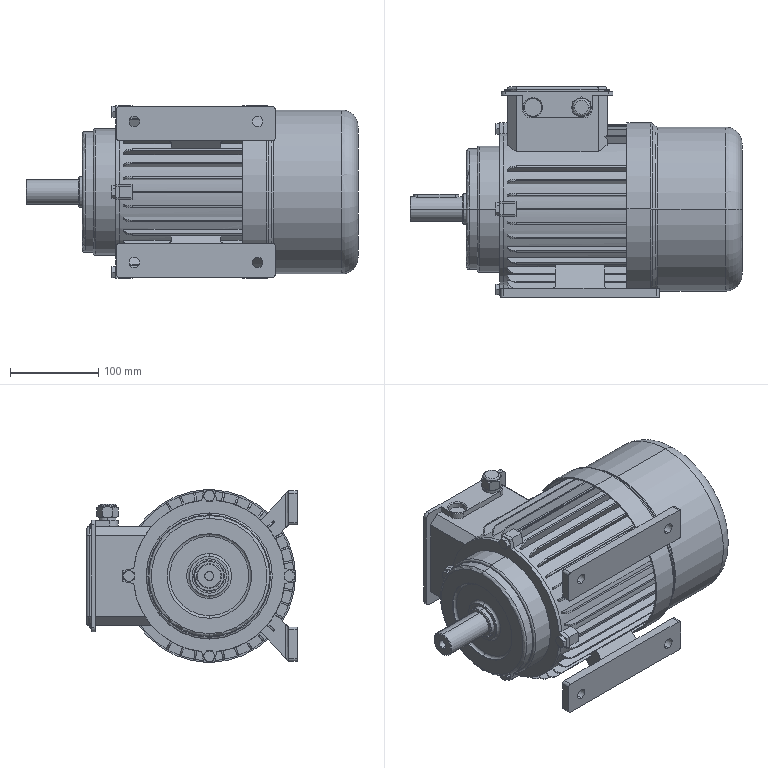Part | STEP file | 3 solids | 638 faces | box 377 x 239.1 x 196 mm | volume 8664532 mm3 | plane 375 | cylinder 165 | cone 48 | torus 46 | sphere 4 | commonest cylinder face diameters 192 x67 6 x20 172.48 x16 5.68 x8 12 x8 20 x8